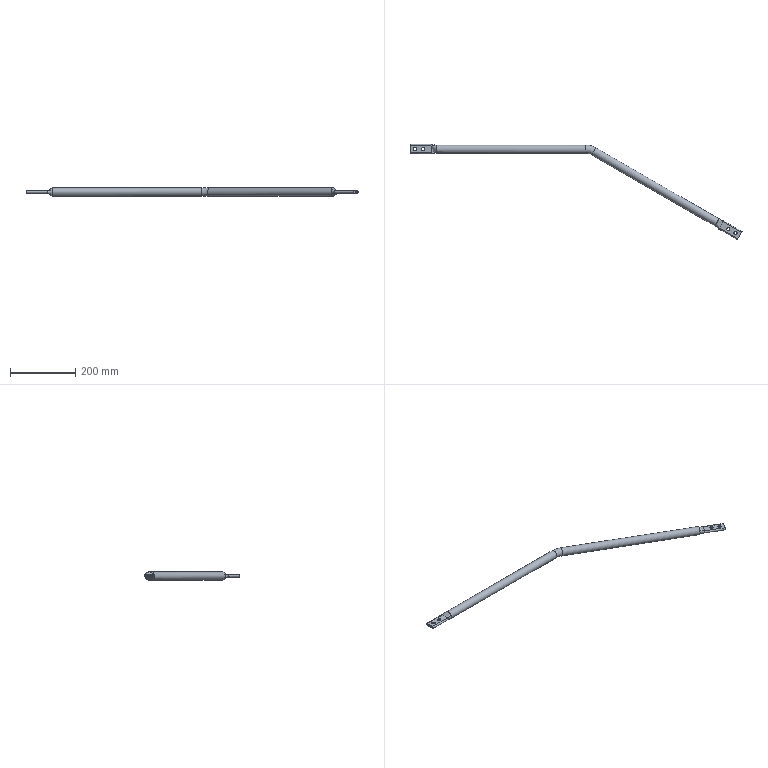Part | STEP file | HL4GZ-1.30.205 (side guard rod 1) | 1 solid | 44 faces | box 1018 x 292.057 x 25 mm | volume 224244 mm3 | cylinder 20 | plane 14 | spline 8 | torus 2 | commonest cylinder face diameters 10 x8 1 x4 7 x4 19 x2 25 x2